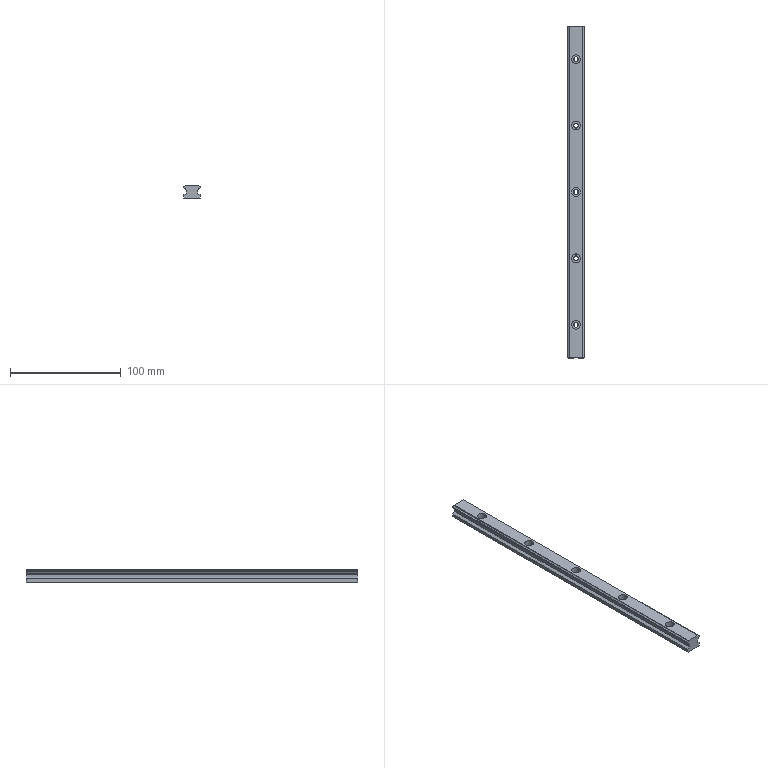Part | STEP file | linear guide EGH15CA-360-30-30_L=360 | 1 solid | 70 faces | box 15 x 300 x 12.5 mm | volume 45472 mm3 | plane 46 | cylinder 24 | commonest cylinder face diameters 4.5 x10 8 x10 3.1 x4